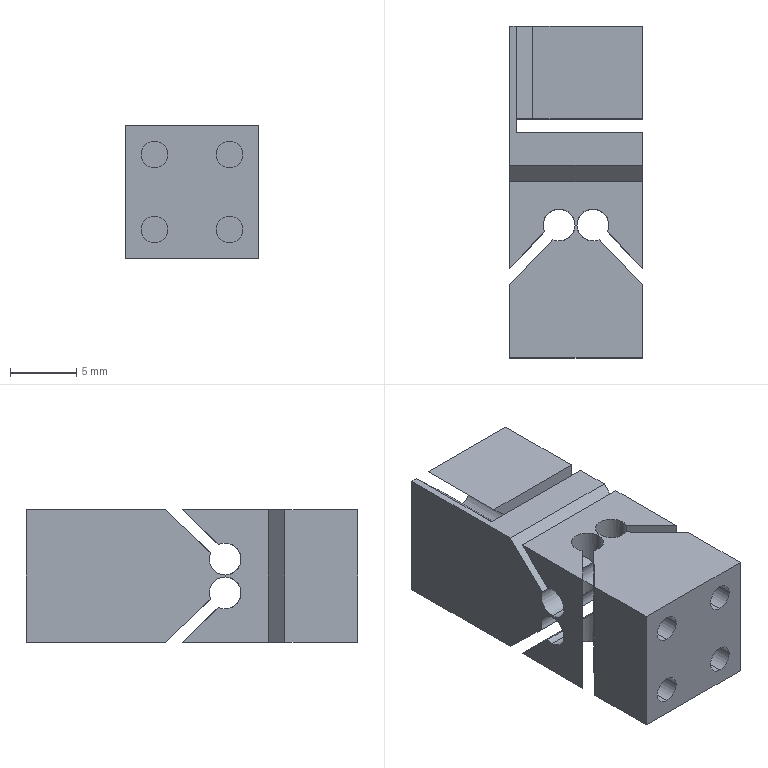Part | SolidWorks | features ICE 8, Extrusion 1 | 1 solid | 96 faces | box 10 x 25 x 10 mm | volume 1930 mm3 | cylinder 62 | plane 34 | commonest cylinder face diameters 2.4 x50 2 x8 1.2 x4